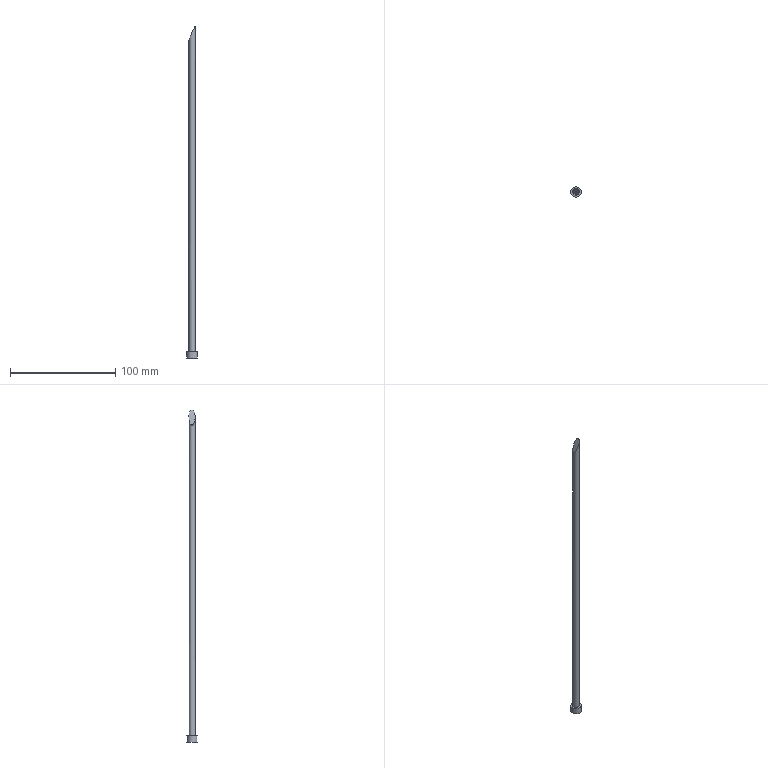Part | NX | features solid 2 | 1 solid | 5 faces | box 10 x 10 x 315.042 mm | volume 9023 mm3 | cylinder 2 | plane 2 | spline 1 | commonest cylinder face diameters 6 x1 10 x1
STEP:
#1=CARTESIAN_POINT('',(-56.,69.,-339.5));
#2=VERTEX_POINT('',#1);
#3=CARTESIAN_POINT('',(-59.,69.,-339.5));
#4=DIRECTION('',(0.,0.,1.));
#5=DIRECTION('',(1.,0.,0.));
#6=AXIS2_PLACEMENT_3D('',#3,#4,#5);
#7=CIRCLE('',#6,3.);
#8=EDGE_CURVE('',#2,#2,#7,.T.);
#9=ORIENTED_EDGE('',*,*,#8,.T.);
#10=EDGE_LOOP('',(#9));
#11=FACE_BOUND('',#10,.T.);
#12=CARTESIAN_POINT('',(-61.981,68.662,-44.637));
#13=VERTEX_POINT('',#12);
#14=CARTESIAN_POINT('',(-61.772,67.789,-43.966));
#15=CARTESIAN_POINT('',(-61.987,68.449,-44.639));
#16=CARTESIAN_POINT('',(-62.011,69.22,-44.768));
#17=CARTESIAN_POINT('',(-61.887,69.92,-44.464));
#18=CARTESIAN_POINT('',(-61.624,70.499,-43.755));
#19=CARTESIAN_POINT('',(-61.278,70.978,-42.825));
#20=CARTESIAN_POINT('',(-60.78,71.453,-41.506));
#21=CARTESIAN_POINT('',(-60.133,71.821,-39.843));
#22=CARTESIAN_POINT('',(-59.303,72.025,-37.805));
#23=CARTESIAN_POINT('',(-58.435,71.99,-35.773));
#24=CARTESIAN_POINT('',(-57.556,71.691,-33.804));
#25=CARTESIAN_POINT('',(-56.8,71.123,-32.183));
#26=CARTESIAN_POINT('',(-56.264,70.317,-31.05));
#27=CARTESIAN_POINT('',(-55.955,69.397,-30.385));
#28=CARTESIAN_POINT('',(-56.041,68.199,-30.482));
#29=CARTESIAN_POINT('',(-56.434,67.387,-31.212));
#30=CARTESIAN_POINT('',(-56.875,66.851,-32.077));
#31=CARTESIAN_POINT('',(-57.492,66.36,-33.337));
#32=CARTESIAN_POINT('',(-58.262,66.044,-34.992));
#33=CARTESIAN_POINT('',(-59.144,65.963,-37.013));
#34=CARTESIAN_POINT('',(-59.973,66.121,-39.037));
#35=CARTESIAN_POINT('',(-60.627,66.447,-40.738));
#36=CARTESIAN_POINT('',(-61.116,66.855,-42.075));
#37=CARTESIAN_POINT('',(-61.461,67.254,-43.05));
#38=CARTESIAN_POINT('',(-61.772,67.789,-43.966));
#39=CARTESIAN_POINT('',(-61.987,68.449,-44.639));
#40=CARTESIAN_POINT('',(-62.011,69.22,-44.768));
#41=B_SPLINE_CURVE_WITH_KNOTS('',3,(#14,#15,#16,#17,#18,#19,#20,#21,#22,#23,#24,#25,#26,#27,#28,#29,#30,#31,#32,#33,#34,#35,#36,#37,#38,#39,#40),.UNSPECIFIED.,.T.,.F.,(1,1,1,1,1,1,1,1,1,1,1,1,1,1,1,1,1,1,1,1,1,1,1,1,1,1,1,1,1,1,1),(-0.003357,-0.002238,-0.001119,0.,0.0005595,0.001119,0.002238,0.003357,0.004476,0.006714,0.008952,0.01119,0.01343,0.01567,0.01679,0.0179,0.01902,0.02014,0.02126,0.02238,0.02462,0.02686,0.02909,0.03133,0.03245,0.03357,0.03469,0.03581,0.03637,0.03693,0.03805),.UNSPECIFIED.);
#42=EDGE_CURVE('',#13,#13,#41,.T.);
#43=ORIENTED_EDGE('',*,*,#42,.T.);
#44=EDGE_LOOP('',(#43));
#45=FACE_BOUND('',#44,.T.);
#46=CARTESIAN_POINT('',(-59.,69.,-345.5));
#47=DIRECTION('',(0.,0.,1.));
#48=DIRECTION('',(1.,0.,0.));
#49=AXIS2_PLACEMENT_3D('',#46,#47,#48);
#50=CYLINDRICAL_SURFACE('',#49,3.);
#51=ADVANCED_FACE('',(#11,#45),#50,.T.);
#52=ORIENTED_EDGE('',*,*,#8,.F.);
#53=EDGE_LOOP('',(#52));
#54=FACE_BOUND('',#53,.T.);
#55=CARTESIAN_POINT('',(-54.,69.,-339.5));
#56=VERTEX_POINT('',#55);
#57=CARTESIAN_POINT('',(-59.,69.,-339.5));
#58=DIRECTION('',(0.,0.,-1.));
#59=DIRECTION('',(1.,0.,0.));
#60=AXIS2_PLACEMENT_3D('',#57,#58,#59);
#61=CIRCLE('',#60,5.);
#62=EDGE_CURVE('',#56,#56,#61,.T.);
#63=ORIENTED_EDGE('',*,*,#62,.F.);
#64=EDGE_LOOP('',(#63));
#65=FACE_BOUND('',#64,.T.);
#66=CARTESIAN_POINT('',(-59.,69.,-339.5));
#67=DIRECTION('',(0.,0.,1.));
#68=DIRECTION('',(1.,0.,0.));
#69=AXIS2_PLACEMENT_3D('',#66,#67,#68);
#70=PLANE('',#69);
#71=ADVANCED_FACE('',(#54,#65),#70,.T.);
#72=CARTESIAN_POINT('',(-54.,69.,-345.5));
#73=VERTEX_POINT('',#72);
#74=CARTESIAN_POINT('',(-59.,69.,-345.5));
#75=DIRECTION('',(0.,0.,1.));
#76=DIRECTION('',(1.,0.,0.));
#77=AXIS2_PLACEMENT_3D('',#74,#75,#76);
#78=CIRCLE('',#77,5.);
#79=EDGE_CURVE('',#73,#73,#78,.T.);
#80=ORIENTED_EDGE('',*,*,#79,.F.);
#81=EDGE_LOOP('',(#80));
#82=FACE_BOUND('',#81,.T.);
#83=CARTESIAN_POINT('',(-59.,69.,-345.5));
#84=DIRECTION('',(0.,0.,-1.));
#85=DIRECTION('',(-1.,0.,0.));
#86=AXIS2_PLACEMENT_3D('',#83,#84,#85);
#87=PLANE('',#86);
#88=ADVANCED_FACE('',(#82),#87,.T.);
#89=ORIENTED_EDGE('',*,*,#62,.T.);
#90=EDGE_LOOP('',(#89));
#91=FACE_BOUND('',#90,.T.);
#92=ORIENTED_EDGE('',*,*,#79,.T.);
#93=EDGE_LOOP('',(#92));
#94=FACE_BOUND('',#93,.T.);
#95=CARTESIAN_POINT('',(-59.,69.,-345.5));
#96=DIRECTION('',(0.,0.,1.));
#97=DIRECTION('',(1.,0.,0.));
#98=AXIS2_PLACEMENT_3D('',#95,#96,#97);
#99=CYLINDRICAL_SURFACE('',#98,5.);
#100=ADVANCED_FACE('',(#91,#94),#99,.T.);
#101=ORIENTED_EDGE('',*,*,#42,.F.);
#102=EDGE_LOOP('',(#101));
#103=FACE_BOUND('',#102,.T.);
#104=CARTESIAN_POINT('',(-62.088,65.843,-44.733));
#105=CARTESIAN_POINT('',(-62.052,67.925,-44.786));
#106=CARTESIAN_POINT('',(-62.014,70.007,-44.839));
#107=CARTESIAN_POINT('',(-61.975,72.089,-44.891));
#108=CARTESIAN_POINT('',(-60.771,65.843,-40.893));
#109=CARTESIAN_POINT('',(-60.734,67.925,-40.946));
#110=CARTESIAN_POINT('',(-60.696,70.007,-40.999));
#111=CARTESIAN_POINT('',(-60.657,72.09,-41.051));
#112=CARTESIAN_POINT('',(-59.268,65.843,-37.121));
#113=CARTESIAN_POINT('',(-59.231,67.925,-37.174));
#114=CARTESIAN_POINT('',(-59.194,70.008,-37.227));
#115=CARTESIAN_POINT('',(-59.155,72.09,-37.279));
#116=CARTESIAN_POINT('',(-57.058,65.843,-32.383));
#117=CARTESIAN_POINT('',(-57.022,67.926,-32.436));
#118=CARTESIAN_POINT('',(-56.985,70.008,-32.488));
#119=CARTESIAN_POINT('',(-56.947,72.09,-32.54));
#120=CARTESIAN_POINT('',(-56.542,65.843,-31.326));
#121=CARTESIAN_POINT('',(-56.507,67.926,-31.379));
#122=CARTESIAN_POINT('',(-56.47,70.008,-31.432));
#123=CARTESIAN_POINT('',(-56.432,72.09,-31.484));
#124=CARTESIAN_POINT('',(-56.008,65.844,-30.279));
#125=CARTESIAN_POINT('',(-55.973,67.926,-30.333));
#126=CARTESIAN_POINT('',(-55.936,70.008,-30.385));
#127=CARTESIAN_POINT('',(-55.898,72.091,-30.437));
#128=B_SPLINE_SURFACE_WITH_KNOTS('',3,3,((#104,#105,#106,#107),(#108,#109,#110,#111),(#112,#113,#114,#115),(#116,#117,#118,#119),(#120,#121,#122,#123),(#124,#125,#126,#127)),.UNSPECIFIED.,.F.,.F.,.F.,(4,2,4),(4,4),(0.1883,0.25,0.2679),(0.8022,0.9208),.UNSPECIFIED.);
#129=ADVANCED_FACE('',(#103),#128,.T.);
#130=CLOSED_SHELL('',(#51,#71,#88,#100,#129));
#131=MANIFOLD_SOLID_BREP('',#130);
#132=(LENGTH_UNIT()NAMED_UNIT(*)SI_UNIT(.MILLI.,.METRE.));
#133=UNCERTAINTY_MEASURE_WITH_UNIT(LENGTH_MEASURE(0.0508),#132,'','');
#134=(NAMED_UNIT(*)PLANE_ANGLE_UNIT()SI_UNIT($,.RADIAN.));
#135=(NAMED_UNIT(*)SI_UNIT($,.STERADIAN.)SOLID_ANGLE_UNIT());
#136=(GEOMETRIC_REPRESENTATION_CONTEXT(3)GLOBAL_UNCERTAINTY_ASSIGNED_CONTEXT((#133))GLOBAL_UNIT_ASSIGNED_CONTEXT((#132,#134,#135))REPRESENTATION_CONTEXT('',''));
#137=ADVANCED_BREP_SHAPE_REPRESENTATION('',(#131),#136);